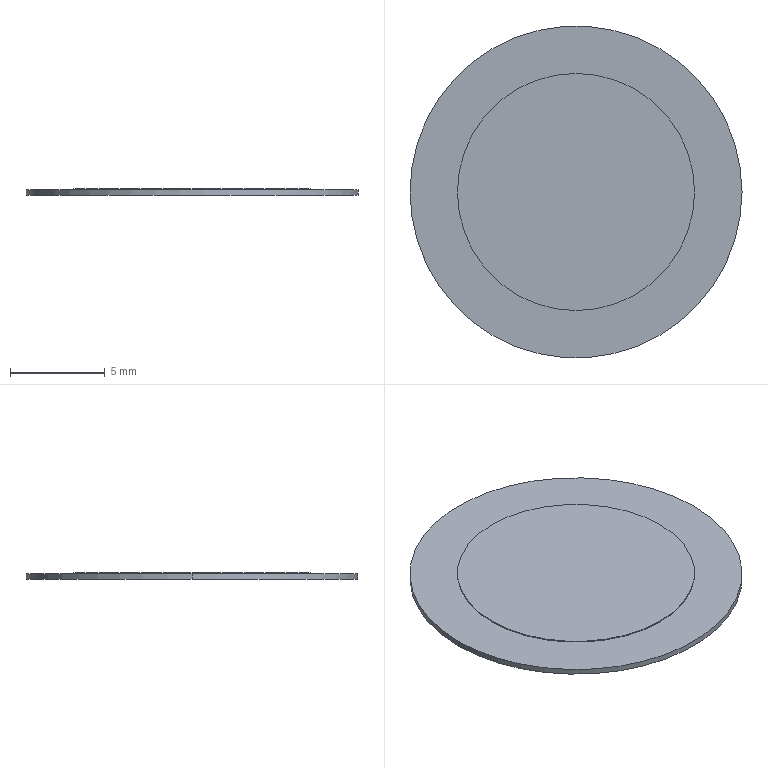Part | SolidWorks | features BaseBody 1, Scale 1 | 1 solid | 7 faces | box 17.5 x 17.5 x 0.35 mm | volume 78.294 mm3 | cylinder 4 | plane 3 | commonest cylinder face diameters 12.5 x2 17.5 x2
STEP:
#1=CARTESIAN_POINT('',(-8.75,0.,0.4637));
#2=VERTEX_POINT('',#1);
#3=CARTESIAN_POINT('',(8.75,0.,0.4637));
#4=VERTEX_POINT('',#3);
#5=CARTESIAN_POINT('',(0.,0.,0.4637));
#6=DIRECTION('',(0.,0.,-1.));
#7=DIRECTION('',(-1.,0.,0.));
#8=AXIS2_PLACEMENT_3D('',#5,#6,#7);
#9=CIRCLE('',#8,8.75);
#10=EDGE_CURVE('',#2,#4,#9,.T.);
#11=ORIENTED_EDGE('',*,*,#10,.T.);
#12=CARTESIAN_POINT('',(8.75,0.,0.1637));
#13=VERTEX_POINT('',#12);
#14=CARTESIAN_POINT('',(8.75,0.,0.4637));
#15=DIRECTION('',(0.,0.,-1.));
#16=VECTOR('',#15,1000.);
#17=LINE('',#14,#16);
#18=EDGE_CURVE('',#4,#13,#17,.T.);
#19=ORIENTED_EDGE('',*,*,#18,.T.);
#20=CARTESIAN_POINT('',(-8.75,0.,0.1637));
#21=VERTEX_POINT('',#20);
#22=CARTESIAN_POINT('',(0.,0.,0.1637));
#23=DIRECTION('',(0.,0.,1.));
#24=DIRECTION('',(-1.,0.,0.));
#25=AXIS2_PLACEMENT_3D('',#22,#23,#24);
#26=CIRCLE('',#25,8.75);
#27=EDGE_CURVE('',#13,#21,#26,.T.);
#28=ORIENTED_EDGE('',*,*,#27,.T.);
#29=CARTESIAN_POINT('',(-8.75,0.,0.4637));
#30=DIRECTION('',(0.,0.,-1.));
#31=VECTOR('',#30,1000.);
#32=LINE('',#29,#31);
#33=EDGE_CURVE('',#2,#21,#32,.T.);
#34=ORIENTED_EDGE('',*,*,#33,.F.);
#35=EDGE_LOOP('',(#11,#19,#28,#34));
#36=FACE_OUTER_BOUND('',#35,.T.);
#37=CARTESIAN_POINT('',(0.,0.,0.4637));
#38=DIRECTION('',(0.,0.,-1.));
#39=DIRECTION('',(-1.,0.,0.));
#40=AXIS2_PLACEMENT_3D('',#37,#38,#39);
#41=CYLINDRICAL_SURFACE('',#40,8.75);
#42=ADVANCED_FACE('',(#36),#41,.T.);
#43=CARTESIAN_POINT('',(-6.25,0.,0.5137));
#44=VERTEX_POINT('',#43);
#45=CARTESIAN_POINT('',(6.25,0.,0.5137));
#46=VERTEX_POINT('',#45);
#47=CARTESIAN_POINT('',(0.,0.,0.5137));
#48=DIRECTION('',(0.,0.,-1.));
#49=DIRECTION('',(-1.,0.,0.));
#50=AXIS2_PLACEMENT_3D('',#47,#48,#49);
#51=CIRCLE('',#50,6.25);
#52=EDGE_CURVE('',#44,#46,#51,.T.);
#53=ORIENTED_EDGE('',*,*,#52,.T.);
#54=CARTESIAN_POINT('',(6.25,0.,0.4637));
#55=VERTEX_POINT('',#54);
#56=CARTESIAN_POINT('',(6.25,0.,0.5137));
#57=DIRECTION('',(0.,0.,-1.));
#58=VECTOR('',#57,1000.);
#59=LINE('',#56,#58);
#60=EDGE_CURVE('',#46,#55,#59,.T.);
#61=ORIENTED_EDGE('',*,*,#60,.T.);
#62=CARTESIAN_POINT('',(-6.25,0.,0.4637));
#63=VERTEX_POINT('',#62);
#64=CARTESIAN_POINT('',(0.,0.,0.4637));
#65=DIRECTION('',(0.,0.,-1.));
#66=DIRECTION('',(-1.,0.,0.));
#67=AXIS2_PLACEMENT_3D('',#64,#65,#66);
#68=CIRCLE('',#67,6.25);
#69=EDGE_CURVE('',#63,#55,#68,.T.);
#70=ORIENTED_EDGE('',*,*,#69,.F.);
#71=CARTESIAN_POINT('',(-6.25,0.,0.5137));
#72=DIRECTION('',(0.,0.,-1.));
#73=VECTOR('',#72,1000.);
#74=LINE('',#71,#73);
#75=EDGE_CURVE('',#44,#63,#74,.T.);
#76=ORIENTED_EDGE('',*,*,#75,.F.);
#77=EDGE_LOOP('',(#53,#61,#70,#76));
#78=FACE_OUTER_BOUND('',#77,.T.);
#79=CARTESIAN_POINT('',(0.,0.,0.5137));
#80=DIRECTION('',(0.,0.,-1.));
#81=DIRECTION('',(-1.,0.,0.));
#82=AXIS2_PLACEMENT_3D('',#79,#80,#81);
#83=CYLINDRICAL_SURFACE('',#82,6.25);
#84=ADVANCED_FACE('',(#78),#83,.T.);
#85=CARTESIAN_POINT('',(0.,0.,0.1637));
#86=DIRECTION('',(0.,0.,1.));
#87=DIRECTION('',(-1.,0.,0.));
#88=AXIS2_PLACEMENT_3D('',#85,#86,#87);
#89=CIRCLE('',#88,8.75);
#90=EDGE_CURVE('',#21,#13,#89,.T.);
#91=ORIENTED_EDGE('',*,*,#90,.F.);
#92=ORIENTED_EDGE('',*,*,#27,.F.);
#93=EDGE_LOOP('',(#91,#92));
#94=FACE_OUTER_BOUND('',#93,.T.);
#95=CARTESIAN_POINT('',(0.,0.,0.1637));
#96=DIRECTION('',(0.,0.,1.));
#97=DIRECTION('',(1.,0.,0.));
#98=AXIS2_PLACEMENT_3D('',#95,#96,#97);
#99=PLANE('',#98);
#100=ADVANCED_FACE('',(#94),#99,.F.);
#101=ORIENTED_EDGE('',*,*,#18,.F.);
#102=CARTESIAN_POINT('',(0.,0.,0.4637));
#103=DIRECTION('',(0.,0.,-1.));
#104=DIRECTION('',(-1.,0.,0.));
#105=AXIS2_PLACEMENT_3D('',#102,#103,#104);
#106=CIRCLE('',#105,8.75);
#107=EDGE_CURVE('',#4,#2,#106,.T.);
#108=ORIENTED_EDGE('',*,*,#107,.T.);
#109=ORIENTED_EDGE('',*,*,#33,.T.);
#110=ORIENTED_EDGE('',*,*,#90,.T.);
#111=EDGE_LOOP('',(#101,#108,#109,#110));
#112=FACE_OUTER_BOUND('',#111,.T.);
#113=CARTESIAN_POINT('',(0.,0.,0.4637));
#114=DIRECTION('',(0.,0.,-1.));
#115=DIRECTION('',(-1.,0.,0.));
#116=AXIS2_PLACEMENT_3D('',#113,#114,#115);
#117=CYLINDRICAL_SURFACE('',#116,8.75);
#118=ADVANCED_FACE('',(#112),#117,.T.);
#119=ORIENTED_EDGE('',*,*,#10,.F.);
#120=ORIENTED_EDGE('',*,*,#107,.F.);
#121=EDGE_LOOP('',(#119,#120));
#122=FACE_OUTER_BOUND('',#121,.T.);
#123=ORIENTED_EDGE('',*,*,#69,.T.);
#124=CARTESIAN_POINT('',(0.,0.,0.4637));
#125=DIRECTION('',(0.,0.,-1.));
#126=DIRECTION('',(-1.,0.,0.));
#127=AXIS2_PLACEMENT_3D('',#124,#125,#126);
#128=CIRCLE('',#127,6.25);
#129=EDGE_CURVE('',#55,#63,#128,.T.);
#130=ORIENTED_EDGE('',*,*,#129,.T.);
#131=EDGE_LOOP('',(#123,#130));
#132=FACE_BOUND('',#131,.T.);
#133=CARTESIAN_POINT('',(0.,0.,0.4637));
#134=DIRECTION('',(0.,0.,1.));
#135=DIRECTION('',(1.,0.,0.));
#136=AXIS2_PLACEMENT_3D('',#133,#134,#135);
#137=PLANE('',#136);
#138=ADVANCED_FACE('',(#122,#132),#137,.T.);
#139=ORIENTED_EDGE('',*,*,#60,.F.);
#140=CARTESIAN_POINT('',(0.,0.,0.5137));
#141=DIRECTION('',(0.,0.,-1.));
#142=DIRECTION('',(-1.,0.,0.));
#143=AXIS2_PLACEMENT_3D('',#140,#141,#142);
#144=CIRCLE('',#143,6.25);
#145=EDGE_CURVE('',#46,#44,#144,.T.);
#146=ORIENTED_EDGE('',*,*,#145,.T.);
#147=ORIENTED_EDGE('',*,*,#75,.T.);
#148=ORIENTED_EDGE('',*,*,#129,.F.);
#149=EDGE_LOOP('',(#139,#146,#147,#148));
#150=FACE_OUTER_BOUND('',#149,.T.);
#151=CARTESIAN_POINT('',(0.,0.,0.5137));
#152=DIRECTION('',(0.,0.,-1.));
#153=DIRECTION('',(-1.,0.,0.));
#154=AXIS2_PLACEMENT_3D('',#151,#152,#153);
#155=CYLINDRICAL_SURFACE('',#154,6.25);
#156=ADVANCED_FACE('',(#150),#155,.T.);
#157=ORIENTED_EDGE('',*,*,#52,.F.);
#158=ORIENTED_EDGE('',*,*,#145,.F.);
#159=EDGE_LOOP('',(#157,#158));
#160=FACE_OUTER_BOUND('',#159,.T.);
#161=CARTESIAN_POINT('',(0.,0.,0.5137));
#162=DIRECTION('',(0.,0.,1.));
#163=DIRECTION('',(1.,0.,0.));
#164=AXIS2_PLACEMENT_3D('',#161,#162,#163);
#165=PLANE('',#164);
#166=ADVANCED_FACE('',(#160),#165,.T.);
#167=CLOSED_SHELL('',(#42,#84,#100,#118,#138,#156,#166));
#168=MANIFOLD_SOLID_BREP('',#167);
#169=CARTESIAN_POINT('',(0.,0.,0.));
#170=DIRECTION('',(0.,0.,1.));
#171=DIRECTION('',(1.,0.,0.));
#172=AXIS2_PLACEMENT_3D('',#169,#170,#171);
#173=(LENGTH_UNIT()NAMED_UNIT(*)SI_UNIT(.MILLI.,.METRE.));
#174=UNCERTAINTY_MEASURE_WITH_UNIT(LENGTH_MEASURE(0.00001),#173,'','');
#175=(NAMED_UNIT(*)PLANE_ANGLE_UNIT()SI_UNIT($,.RADIAN.));
#176=(NAMED_UNIT(*)SI_UNIT($,.STERADIAN.)SOLID_ANGLE_UNIT());
#177=(GEOMETRIC_REPRESENTATION_CONTEXT(3)GLOBAL_UNCERTAINTY_ASSIGNED_CONTEXT((#174))GLOBAL_UNIT_ASSIGNED_CONTEXT((#173,#175,#176))REPRESENTATION_CONTEXT('',''));
#178=ADVANCED_BREP_SHAPE_REPRESENTATION('',(#168,#172),#177);